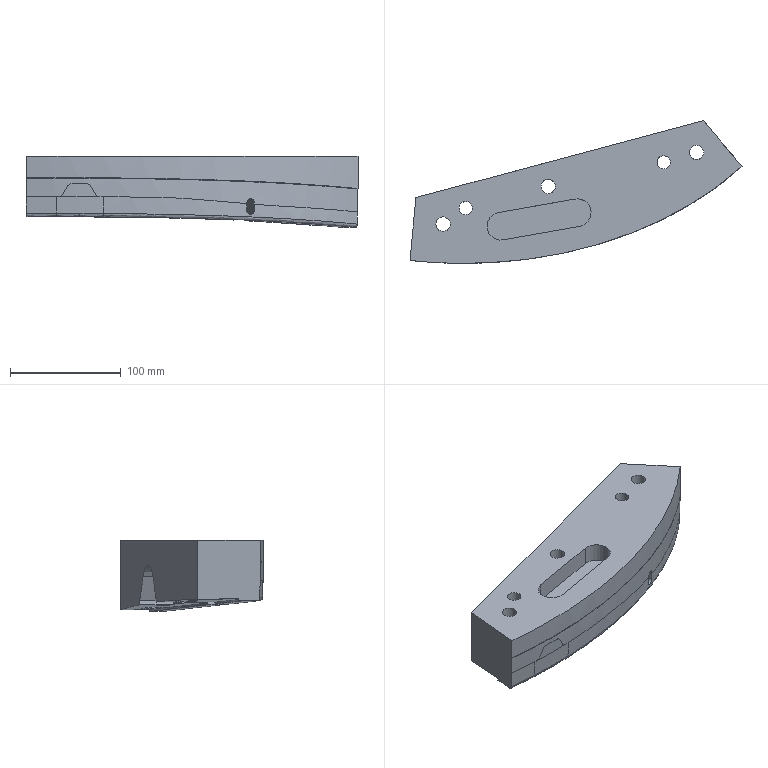Part | NX | features solid 2 | 1 solid | 69 faces | box 299.601 x 128.906 x 64.174 mm | volume 1055176 mm3 | spline 26 | plane 22 | cylinder 18 | sphere 2 | cone 1 | commonest cylinder face diameters 10 x5 13 x3 20 x3 7.1 x2 12 x2 25 x2